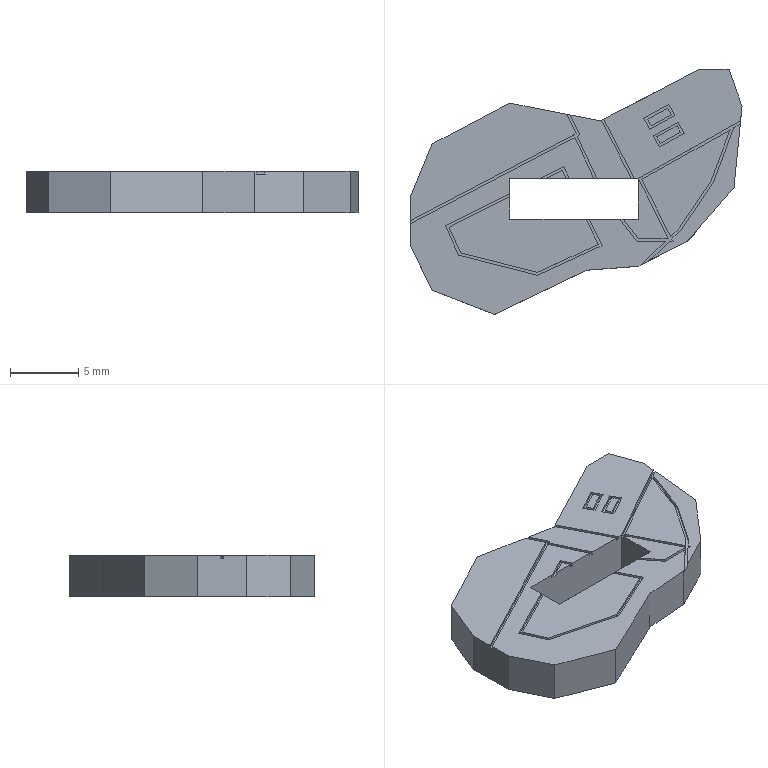Part | SolidWorks | features BaseBody 1 | 1 solid | 100 faces | box 24.24 x 17.887 x 3 mm | volume 761.054 mm3 | plane 86 | spline 14